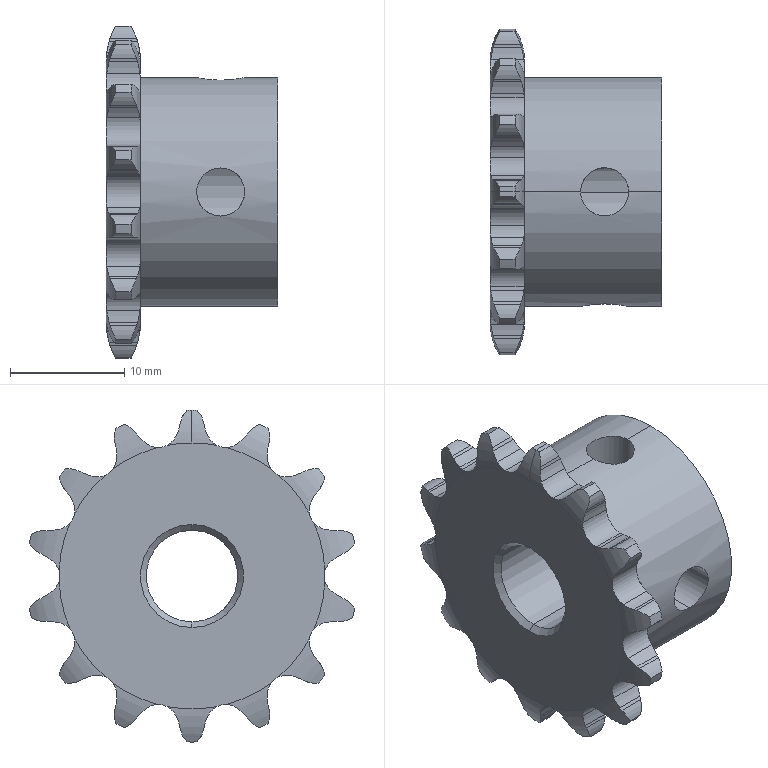Part | SolidWorks | features ICE 3, CirPattern 2, Chamfer 1, Cut 1, HoleWzd 1, RefAxis 1, Revolution 1 | 1 solid | 164 faces | box 15 x 28.455 x 29 mm | volume 4351 mm3 | cylinder 99 | plane 31 | torus 30 | cone 4 | commonest cylinder face diameters 4.824 x30 8.696 x28 3.416 x18 29 x15 4.2 x4 8 x2